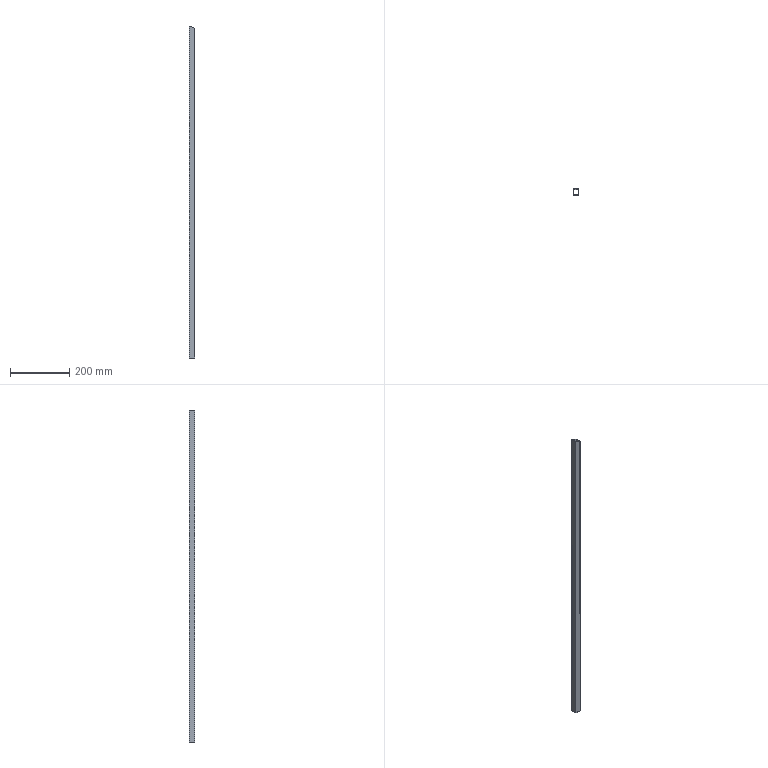Part | NX | features BREP 1 | 1 solid | 10 faces | box 20 x 20 x 1122 mm | volume 161028 mm3 | plane 10
STEP:
#1=CARTESIAN_POINT('',(775.673,680.,1223.936));
#2=VERTEX_POINT('',#1);
#3=CARTESIAN_POINT('',(759.673,680.,1230.563));
#4=VERTEX_POINT('',#3);
#5=CARTESIAN_POINT('',(767.673,680.,1227.25));
#6=DIRECTION('',(-0.9239,0.,0.3827));
#7=VECTOR('',#6,1000.);
#8=LINE('',#5,#7);
#9=EDGE_CURVE('',#2,#4,#8,.T.);
#10=ORIENTED_EDGE('',*,*,#9,.T.);
#11=CARTESIAN_POINT('',(759.673,696.,1230.563));
#12=VERTEX_POINT('',#11);
#13=CARTESIAN_POINT('',(759.673,688.,1230.563));
#14=DIRECTION('',(0.,-1.,0.));
#15=VECTOR('',#14,1000.);
#16=LINE('',#13,#15);
#17=EDGE_CURVE('',#12,#4,#16,.T.);
#18=ORIENTED_EDGE('',*,*,#17,.F.);
#19=CARTESIAN_POINT('',(775.673,696.,1223.936));
#20=VERTEX_POINT('',#19);
#21=CARTESIAN_POINT('',(767.673,696.,1227.25));
#22=DIRECTION('',(-0.9239,0.,0.3827));
#23=VECTOR('',#22,1000.);
#24=LINE('',#21,#23);
#25=EDGE_CURVE('',#20,#12,#24,.T.);
#26=ORIENTED_EDGE('',*,*,#25,.F.);
#27=CARTESIAN_POINT('',(775.673,696.,1223.936));
#28=CARTESIAN_POINT('',(775.673,680.,1223.936));
#29=B_SPLINE_CURVE_WITH_KNOTS('',1,(#27,#28),.UNSPECIFIED.,.F.,.F.,(2,2),(2.,18.),.UNSPECIFIED.);
#30=EDGE_CURVE('',#20,#2,#29,.T.);
#31=ORIENTED_EDGE('',*,*,#30,.T.);
#32=EDGE_LOOP('',(#10,#18,#26,#31));
#33=FACE_BOUND('',#32,.T.);
#34=CARTESIAN_POINT('',(757.673,698.,1231.392));
#35=VERTEX_POINT('',#34);
#36=CARTESIAN_POINT('',(757.673,678.,1231.392));
#37=VERTEX_POINT('',#36);
#38=CARTESIAN_POINT('',(757.673,688.,1231.392));
#39=DIRECTION('',(0.,-1.,0.));
#40=VECTOR('',#39,1000.);
#41=LINE('',#38,#40);
#42=EDGE_CURVE('',#35,#37,#41,.T.);
#43=ORIENTED_EDGE('',*,*,#42,.T.);
#44=CARTESIAN_POINT('',(777.673,678.,1223.108));
#45=VERTEX_POINT('',#44);
#46=CARTESIAN_POINT('',(767.673,678.,1227.25));
#47=DIRECTION('',(0.9239,0.,-0.3827));
#48=VECTOR('',#47,1000.);
#49=LINE('',#46,#48);
#50=EDGE_CURVE('',#37,#45,#49,.T.);
#51=ORIENTED_EDGE('',*,*,#50,.T.);
#52=CARTESIAN_POINT('',(777.673,698.,1223.108));
#53=VERTEX_POINT('',#52);
#54=CARTESIAN_POINT('',(777.673,698.,1223.108));
#55=CARTESIAN_POINT('',(777.673,694.,1223.108));
#56=CARTESIAN_POINT('',(777.673,690.,1223.108));
#57=CARTESIAN_POINT('',(777.673,686.,1223.108));
#58=CARTESIAN_POINT('',(777.673,682.,1223.108));
#59=CARTESIAN_POINT('',(777.673,678.,1223.108));
#60=B_SPLINE_CURVE_WITH_KNOTS('',5,(#54,#55,#56,#57,#58,#59),.UNSPECIFIED.,.F.,.F.,(6,6),(0.,20.),.UNSPECIFIED.);
#61=EDGE_CURVE('',#53,#45,#60,.T.);
#62=ORIENTED_EDGE('',*,*,#61,.F.);
#63=CARTESIAN_POINT('',(767.673,698.,1227.25));
#64=DIRECTION('',(0.9239,0.,-0.3827));
#65=VECTOR('',#64,1000.);
#66=LINE('',#63,#65);
#67=EDGE_CURVE('',#35,#53,#66,.T.);
#68=ORIENTED_EDGE('',*,*,#67,.F.);
#69=EDGE_LOOP('',(#43,#51,#62,#68));
#70=FACE_BOUND('',#69,.T.);
#71=CARTESIAN_POINT('',(757.673,678.,1231.392));
#72=DIRECTION('',(0.3827,0.,0.9239));
#73=DIRECTION('',(0.9239,0.,-0.3827));
#74=AXIS2_PLACEMENT_3D('',#71,#72,#73);
#75=PLANE('',#74);
#76=ADVANCED_FACE('',(#33,#70),#75,.T.);
#77=ORIENTED_EDGE('',*,*,#30,.F.);
#78=CARTESIAN_POINT('',(775.673,696.,109.));
#79=VERTEX_POINT('',#78);
#80=CARTESIAN_POINT('',(775.673,696.,666.468));
#81=DIRECTION('',(0.,0.,1.));
#82=VECTOR('',#81,1000.);
#83=LINE('',#80,#82);
#84=EDGE_CURVE('',#79,#20,#83,.T.);
#85=ORIENTED_EDGE('',*,*,#84,.F.);
#86=CARTESIAN_POINT('',(775.673,680.,109.));
#87=VERTEX_POINT('',#86);
#88=CARTESIAN_POINT('',(775.673,688.,109.));
#89=DIRECTION('',(0.,-1.,0.));
#90=VECTOR('',#89,1000.);
#91=LINE('',#88,#90);
#92=EDGE_CURVE('',#79,#87,#91,.T.);
#93=ORIENTED_EDGE('',*,*,#92,.T.);
#94=CARTESIAN_POINT('',(775.673,680.,666.468));
#95=DIRECTION('',(0.,0.,1.));
#96=VECTOR('',#95,1000.);
#97=LINE('',#94,#96);
#98=EDGE_CURVE('',#87,#2,#97,.T.);
#99=ORIENTED_EDGE('',*,*,#98,.T.);
#100=EDGE_LOOP('',(#77,#85,#93,#99));
#101=FACE_BOUND('',#100,.T.);
#102=CARTESIAN_POINT('',(775.673,688.,666.468));
#103=DIRECTION('',(1.,0.,0.));
#104=DIRECTION('',(0.,0.,-1.));
#105=AXIS2_PLACEMENT_3D('',#102,#103,#104);
#106=PLANE('',#105);
#107=ADVANCED_FACE('',(#101),#106,.F.);
#108=ORIENTED_EDGE('',*,*,#9,.F.);
#109=ORIENTED_EDGE('',*,*,#98,.F.);
#110=CARTESIAN_POINT('',(759.673,680.,109.));
#111=VERTEX_POINT('',#110);
#112=CARTESIAN_POINT('',(767.673,680.,109.));
#113=DIRECTION('',(1.,0.,0.));
#114=VECTOR('',#113,1000.);
#115=LINE('',#112,#114);
#116=EDGE_CURVE('',#111,#87,#115,.T.);
#117=ORIENTED_EDGE('',*,*,#116,.F.);
#118=CARTESIAN_POINT('',(759.673,680.,669.782));
#119=DIRECTION('',(0.,0.,-1.));
#120=VECTOR('',#119,1000.);
#121=LINE('',#118,#120);
#122=EDGE_CURVE('',#4,#111,#121,.T.);
#123=ORIENTED_EDGE('',*,*,#122,.F.);
#124=EDGE_LOOP('',(#108,#109,#117,#123));
#125=FACE_BOUND('',#124,.T.);
#126=CARTESIAN_POINT('',(757.673,680.,1249.127));
#127=DIRECTION('',(0.,-1.,0.));
#128=DIRECTION('',(0.,0.,-1.));
#129=AXIS2_PLACEMENT_3D('',#126,#127,#128);
#130=PLANE('',#129);
#131=ADVANCED_FACE('',(#125),#130,.F.);
#132=ORIENTED_EDGE('',*,*,#17,.T.);
#133=ORIENTED_EDGE('',*,*,#122,.T.);
#134=CARTESIAN_POINT('',(759.673,696.,109.));
#135=VERTEX_POINT('',#134);
#136=CARTESIAN_POINT('',(759.673,688.,109.));
#137=DIRECTION('',(0.,-1.,0.));
#138=VECTOR('',#137,1000.);
#139=LINE('',#136,#138);
#140=EDGE_CURVE('',#135,#111,#139,.T.);
#141=ORIENTED_EDGE('',*,*,#140,.F.);
#142=CARTESIAN_POINT('',(759.673,696.,669.782));
#143=DIRECTION('',(0.,0.,-1.));
#144=VECTOR('',#143,1000.);
#145=LINE('',#142,#144);
#146=EDGE_CURVE('',#12,#135,#145,.T.);
#147=ORIENTED_EDGE('',*,*,#146,.F.);
#148=EDGE_LOOP('',(#132,#133,#141,#147));
#149=FACE_BOUND('',#148,.T.);
#150=CARTESIAN_POINT('',(759.673,698.,1249.127));
#151=DIRECTION('',(-1.,0.,0.));
#152=DIRECTION('',(0.,0.,-1.));
#153=AXIS2_PLACEMENT_3D('',#150,#151,#152);
#154=PLANE('',#153);
#155=ADVANCED_FACE('',(#149),#154,.F.);
#156=ORIENTED_EDGE('',*,*,#146,.T.);
#157=CARTESIAN_POINT('',(767.673,696.,109.));
#158=DIRECTION('',(1.,0.,0.));
#159=VECTOR('',#158,1000.);
#160=LINE('',#157,#159);
#161=EDGE_CURVE('',#135,#79,#160,.T.);
#162=ORIENTED_EDGE('',*,*,#161,.T.);
#163=ORIENTED_EDGE('',*,*,#84,.T.);
#164=ORIENTED_EDGE('',*,*,#25,.T.);
#165=EDGE_LOOP('',(#156,#162,#163,#164));
#166=FACE_BOUND('',#165,.T.);
#167=CARTESIAN_POINT('',(757.673,696.,1249.127));
#168=DIRECTION('',(0.,-1.,0.));
#169=DIRECTION('',(0.,0.,-1.));
#170=AXIS2_PLACEMENT_3D('',#167,#168,#169);
#171=PLANE('',#170);
#172=ADVANCED_FACE('',(#166),#171,.T.);
#173=CARTESIAN_POINT('',(777.673,678.,109.));
#174=VERTEX_POINT('',#173);
#175=CARTESIAN_POINT('',(777.673,678.,666.054));
#176=DIRECTION('',(0.,0.,-1.));
#177=VECTOR('',#176,1000.);
#178=LINE('',#175,#177);
#179=EDGE_CURVE('',#45,#174,#178,.T.);
#180=ORIENTED_EDGE('',*,*,#179,.T.);
#181=CARTESIAN_POINT('',(777.673,698.,109.));
#182=VERTEX_POINT('',#181);
#183=CARTESIAN_POINT('',(777.673,688.,109.));
#184=DIRECTION('',(0.,-1.,0.));
#185=VECTOR('',#184,1000.);
#186=LINE('',#183,#185);
#187=EDGE_CURVE('',#182,#174,#186,.T.);
#188=ORIENTED_EDGE('',*,*,#187,.F.);
#189=CARTESIAN_POINT('',(777.673,698.,666.054));
#190=DIRECTION('',(0.,0.,-1.));
#191=VECTOR('',#190,1000.);
#192=LINE('',#189,#191);
#193=EDGE_CURVE('',#53,#182,#192,.T.);
#194=ORIENTED_EDGE('',*,*,#193,.F.);
#195=ORIENTED_EDGE('',*,*,#61,.T.);
#196=EDGE_LOOP('',(#180,#188,#194,#195));
#197=FACE_BOUND('',#196,.T.);
#198=CARTESIAN_POINT('',(777.673,688.,598.034));
#199=DIRECTION('',(1.,0.,0.));
#200=DIRECTION('',(0.,0.,-1.));
#201=AXIS2_PLACEMENT_3D('',#198,#199,#200);
#202=PLANE('',#201);
#203=ADVANCED_FACE('',(#197),#202,.T.);
#204=ORIENTED_EDGE('',*,*,#67,.T.);
#205=ORIENTED_EDGE('',*,*,#193,.T.);
#206=CARTESIAN_POINT('',(757.673,698.,109.));
#207=VERTEX_POINT('',#206);
#208=CARTESIAN_POINT('',(767.673,698.,109.));
#209=DIRECTION('',(1.,0.,0.));
#210=VECTOR('',#209,1000.);
#211=LINE('',#208,#210);
#212=EDGE_CURVE('',#207,#182,#211,.T.);
#213=ORIENTED_EDGE('',*,*,#212,.F.);
#214=CARTESIAN_POINT('',(757.673,698.,670.196));
#215=DIRECTION('',(0.,0.,-1.));
#216=VECTOR('',#215,1000.);
#217=LINE('',#214,#216);
#218=EDGE_CURVE('',#35,#207,#217,.T.);
#219=ORIENTED_EDGE('',*,*,#218,.F.);
#220=EDGE_LOOP('',(#204,#205,#213,#219));
#221=FACE_BOUND('',#220,.T.);
#222=CARTESIAN_POINT('',(757.673,698.,1249.127));
#223=DIRECTION('',(0.,-1.,0.));
#224=DIRECTION('',(0.,0.,-1.));
#225=AXIS2_PLACEMENT_3D('',#222,#223,#224);
#226=PLANE('',#225);
#227=ADVANCED_FACE('',(#221),#226,.F.);
#228=ORIENTED_EDGE('',*,*,#218,.T.);
#229=CARTESIAN_POINT('',(757.673,678.,109.));
#230=VERTEX_POINT('',#229);
#231=CARTESIAN_POINT('',(757.673,688.,109.));
#232=DIRECTION('',(0.,-1.,0.));
#233=VECTOR('',#232,1000.);
#234=LINE('',#231,#233);
#235=EDGE_CURVE('',#207,#230,#234,.T.);
#236=ORIENTED_EDGE('',*,*,#235,.T.);
#237=CARTESIAN_POINT('',(757.673,678.,670.196));
#238=DIRECTION('',(0.,0.,-1.));
#239=VECTOR('',#238,1000.);
#240=LINE('',#237,#239);
#241=EDGE_CURVE('',#37,#230,#240,.T.);
#242=ORIENTED_EDGE('',*,*,#241,.F.);
#243=ORIENTED_EDGE('',*,*,#42,.F.);
#244=EDGE_LOOP('',(#228,#236,#242,#243));
#245=FACE_BOUND('',#244,.T.);
#246=CARTESIAN_POINT('',(757.673,698.,1249.127));
#247=DIRECTION('',(-1.,0.,0.));
#248=DIRECTION('',(0.,0.,-1.));
#249=AXIS2_PLACEMENT_3D('',#246,#247,#248);
#250=PLANE('',#249);
#251=ADVANCED_FACE('',(#245),#250,.T.);
#252=ORIENTED_EDGE('',*,*,#241,.T.);
#253=CARTESIAN_POINT('',(767.673,678.,109.));
#254=DIRECTION('',(1.,0.,0.));
#255=VECTOR('',#254,1000.);
#256=LINE('',#253,#255);
#257=EDGE_CURVE('',#230,#174,#256,.T.);
#258=ORIENTED_EDGE('',*,*,#257,.T.);
#259=ORIENTED_EDGE('',*,*,#179,.F.);
#260=ORIENTED_EDGE('',*,*,#50,.F.);
#261=EDGE_LOOP('',(#252,#258,#259,#260));
#262=FACE_BOUND('',#261,.T.);
#263=CARTESIAN_POINT('',(757.673,678.,1249.127));
#264=DIRECTION('',(0.,-1.,0.));
#265=DIRECTION('',(0.,0.,-1.));
#266=AXIS2_PLACEMENT_3D('',#263,#264,#265);
#267=PLANE('',#266);
#268=ADVANCED_FACE('',(#262),#267,.T.);
#269=ORIENTED_EDGE('',*,*,#161,.F.);
#270=ORIENTED_EDGE('',*,*,#140,.T.);
#271=ORIENTED_EDGE('',*,*,#116,.T.);
#272=ORIENTED_EDGE('',*,*,#92,.F.);
#273=EDGE_LOOP('',(#269,#270,#271,#272));
#274=FACE_BOUND('',#273,.T.);
#275=ORIENTED_EDGE('',*,*,#257,.F.);
#276=ORIENTED_EDGE('',*,*,#235,.F.);
#277=ORIENTED_EDGE('',*,*,#212,.T.);
#278=ORIENTED_EDGE('',*,*,#187,.T.);
#279=EDGE_LOOP('',(#275,#276,#277,#278));
#280=FACE_BOUND('',#279,.T.);
#281=CARTESIAN_POINT('',(687.53,698.,109.));
#282=DIRECTION('',(0.,0.,-1.));
#283=DIRECTION('',(1.,0.,0.));
#284=AXIS2_PLACEMENT_3D('',#281,#282,#283);
#285=PLANE('',#284);
#286=ADVANCED_FACE('',(#274,#280),#285,.T.);
#287=CLOSED_SHELL('',(#76,#107,#131,#155,#172,#203,#227,#251,#268,#286));
#288=MANIFOLD_SOLID_BREP('',#287);
#289=(LENGTH_UNIT()NAMED_UNIT(*)SI_UNIT(.MILLI.,.METRE.));
#290=UNCERTAINTY_MEASURE_WITH_UNIT(LENGTH_MEASURE(0.00001),#289,'','');
#291=(NAMED_UNIT(*)PLANE_ANGLE_UNIT()SI_UNIT($,.RADIAN.));
#292=(NAMED_UNIT(*)SI_UNIT($,.STERADIAN.)SOLID_ANGLE_UNIT());
#293=(GEOMETRIC_REPRESENTATION_CONTEXT(3)GLOBAL_UNCERTAINTY_ASSIGNED_CONTEXT((#290))GLOBAL_UNIT_ASSIGNED_CONTEXT((#289,#291,#292))REPRESENTATION_CONTEXT('',''));
#294=ADVANCED_BREP_SHAPE_REPRESENTATION('',(#288),#293);